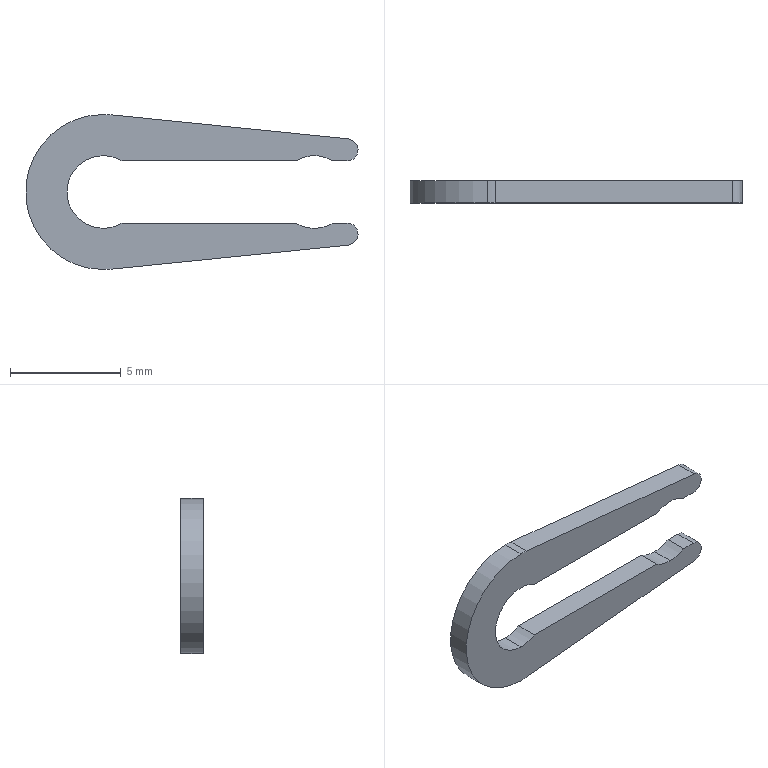Part | STEP file | 06B side guide chain buckle | 1 solid | 19 faces | box 15 x 1 x 7 mm | volume 49.292 mm3 | cylinder 11 | plane 8 | commonest cylinder face diameters 3.28 x6 7 x3 1 x2